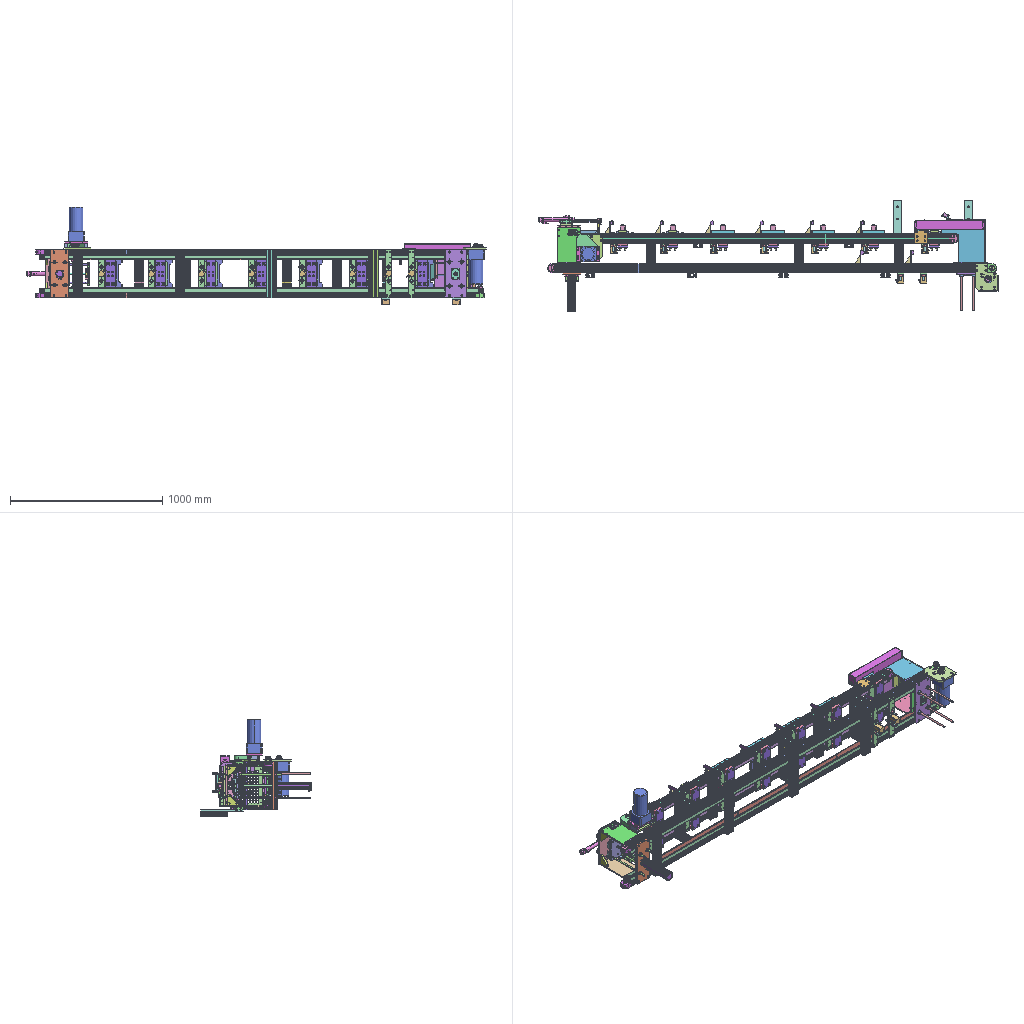Assembly | STEP file | 130 different items | 544 placed | box 3024 x 734 x 644 mm
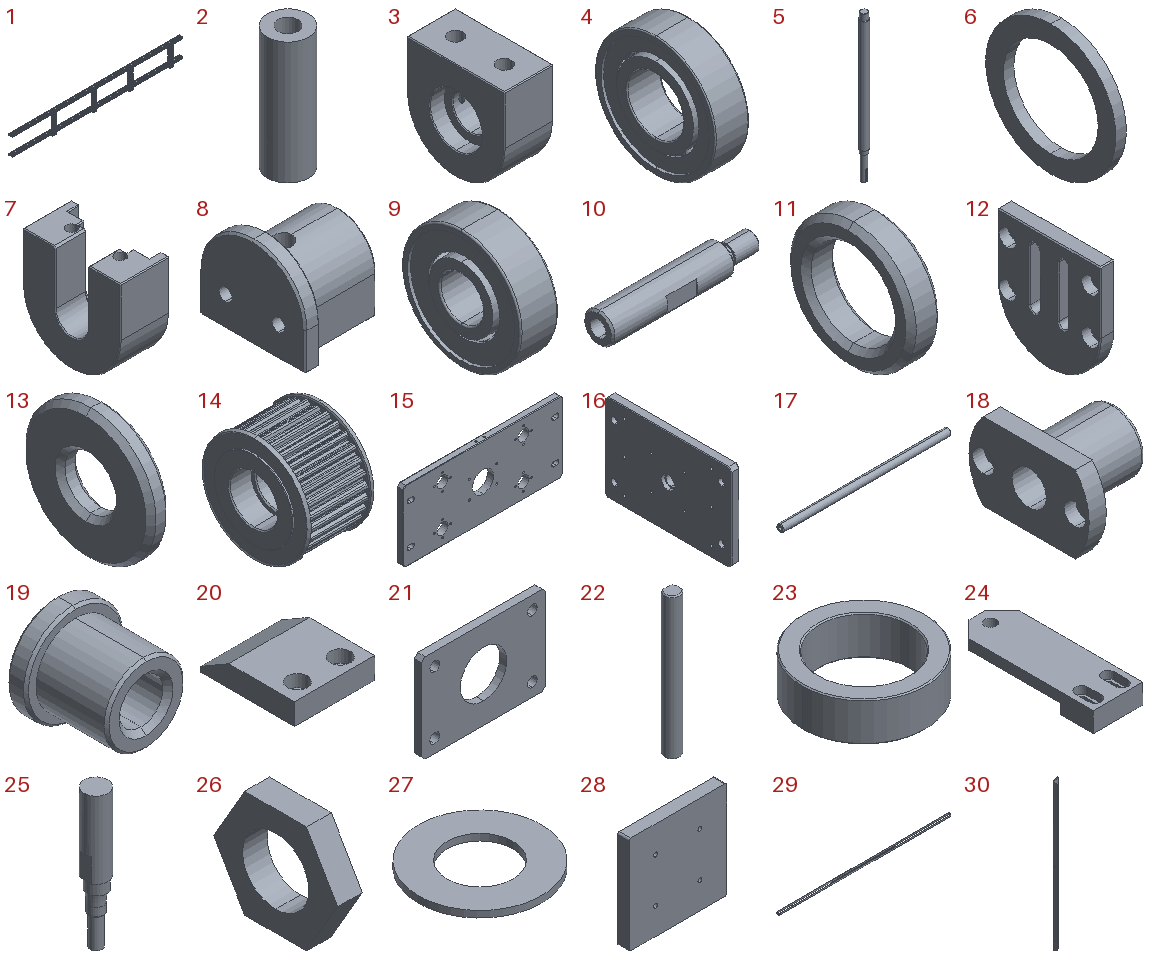Parts list (item | name | quantity | parent item | size | volume):
1 | Welding Conveyor Frame_Default<As Machined> | x1 | in BPSP-03Fixture Return Conveyor Assembly_Default | 2830 x 90 x 316 mm | 3898026 mm3
2 | DYCS-M-15-17 Threaded Bushing_Default | x16 | in BPSP-03Fixture Return Conveyor Assembly_Default, BPSP-02Welding Conveyor Assembly_Default | 10 x 10 x 30 mm | 1767 mm3
3 | BPSP-03-004 Elevator Drive Shaft Fixing Plate_Default | x4 | in BPSP-03Fixture Return Conveyor Assembly_Default, BPSP-02Welding Conveyor Assembly_Default | 30 x 60 x 60 mm | 72459 mm3
4 | GB/T276-94Deep Groove Ball Bearing6002-2Z | x4 | in BPSP-03Fixture Return Conveyor Assembly_Default, BPSP-02Welding Conveyor Assembly_Default | 9 x 32 x 32 mm | 3545 mm3
5 | BPSP-03-006 Drive Shaft_Default | x2 | in BPSP-03Fixture Return Conveyor Assembly_Default, BPSP-02Welding Conveyor Assembly_Default | 18 x 18 x 335 mm | 73475 mm3
6 | BPSP-03-005 Locating Ring_Default | x4 | in BPSP-03Fixture Return Conveyor Assembly_Default, BPSP-02Welding Conveyor Assembly_Default | 2 x 25 x 25 mm | 461.437 mm3
7 | BPSP-03-018 Driven Wheel Mounting Plate_Default | x4 | in Driven Wheel Assembly_Default | 30 x 60 x 60 mm | 50936 mm3
8 | BPSP-03-019 Driven Wheel Fixing Block_Default | x4 | in Driven Wheel Assembly_Default | 23 x 28 x 24 mm | 8364 mm3
9 | GB/T276-94Deep Groove Ball Bearing608-2Z | x8 | in Driven Wheel Assembly_Default | 7 x 22 x 22 mm | 1460 mm3
10 | BPSP-03-021 Fixed Shaft_Default | x4 | in Driven Wheel Assembly_Default | 40.5 x 8 x 8 mm | 1575 mm3
11 | BPSP-03-022 Driven Wheel Stop Washer_Default | x4 | in Driven Wheel Assembly_Default | 3 x 12 x 12 mm | 168.916 mm3
12 | BPSP-03-020 Clamp Block_Default | x4 | in Driven Wheel Assembly_Default | 7 x 50 x 55 mm | 14443 mm3
13 | BPSP-03-023 Driven Wheel Fixing Washer_Default | x4 | in Driven Wheel Assembly_Default | 2 x 13 x 13 mm | 208.696 mm3
14 | BPSP-03-032 T5Timing Pulley30 Tooth2 | x4 | in Driven Wheel Assembly_Default | 32 x 49 x 49 mm | 40684 mm3
15 | BPSP-03-012 Linear Bearing Mounting Plate_Default | x1 | in Elevator Lift Mechanism | 316 x 12 x 140 mm | 486609 mm3
16 | BPSP-03-013 Test Station Lift Plate_Default | x1 | in Elevator Lift Mechanism | 12 x 190 x 130 mm | 287114 mm3
17 | BPSP-03-016 Lift Chrome Rod_Default | x4 | in Elevator Lift Mechanism | 280 x 12 x 12 mm | 31385 mm3
18 | LHFC12_LHFC12 | x4 | in Elevator Lift Mechanism | 30 x 42 x 27 mm | 10763 mm3
19 | BPSP-03-039Lift Joint | x1 | in Elevator Lift Mechanism | 19.8 x 18 x 19.8 mm | 2819 mm3
20 | BPSP-03-015 Shaft Pivot Seat | x2 | in Elevator Lift Mechanism | 30 x 35 x 8 mm | 6950 mm3
21 | BPSP-03-038Support Cylinder Fixing Plate_Default | x1 | in Elevator Lift Mechanism | 70 x 4 x 50 mm | 11431 mm3
22 | BPSP-03-014 Sliding Rib_Default | x2 | in Elevator Lift Mechanism | 14 x 12 x 130 mm | 17958 mm3
23 | BPSP-03-037Lift Retaining Ring_Default | x1 | in Elevator Lift Mechanism | 22 x 22 x 7 mm | 1249 mm3
24 | BPSP-03-036Proximity Switch Mounting Plate | x1 | in Elevator Lift Mechanism | 30 x 85 x 12 mm | 16342 mm3
25 | E2E_X2D1_N_BASE | x1 | in Proximity SensorE2E_X2D1_N | 8 x 8 x 47 mm | 1680 mm3
26 | E2E_X2D1_N_NUT | x2 | in Proximity SensorE2E_X2D1_N | 3 x 15.011 x 13 mm | 288.278 mm3
27 | E2E_X2D1_N_WASHER | x1 | in Proximity SensorE2E_X2D1_N | 15 x 15 x 0.8 mm | 101.159 mm3
28 | Ejector Urethane Pad_Default | x1 | in Elevator Lift Mechanism | 110 x 13 x 110 mm | 155824 mm3
29 | Belt1-11^BPSP-03Fixture Return Conveyor Assembly_Default | x2 | in BPSP-03Fixture Return Conveyor Assembly_Default | 2922 x 49 x 25 mm | 294683 mm3
30 | BPSP-03-031Long Support Plate (Lower)_Default | x6 | in BPSP-03Fixture Return Conveyor Assembly_Default | 35 x 30 x 929.978 mm | 113908 mm3
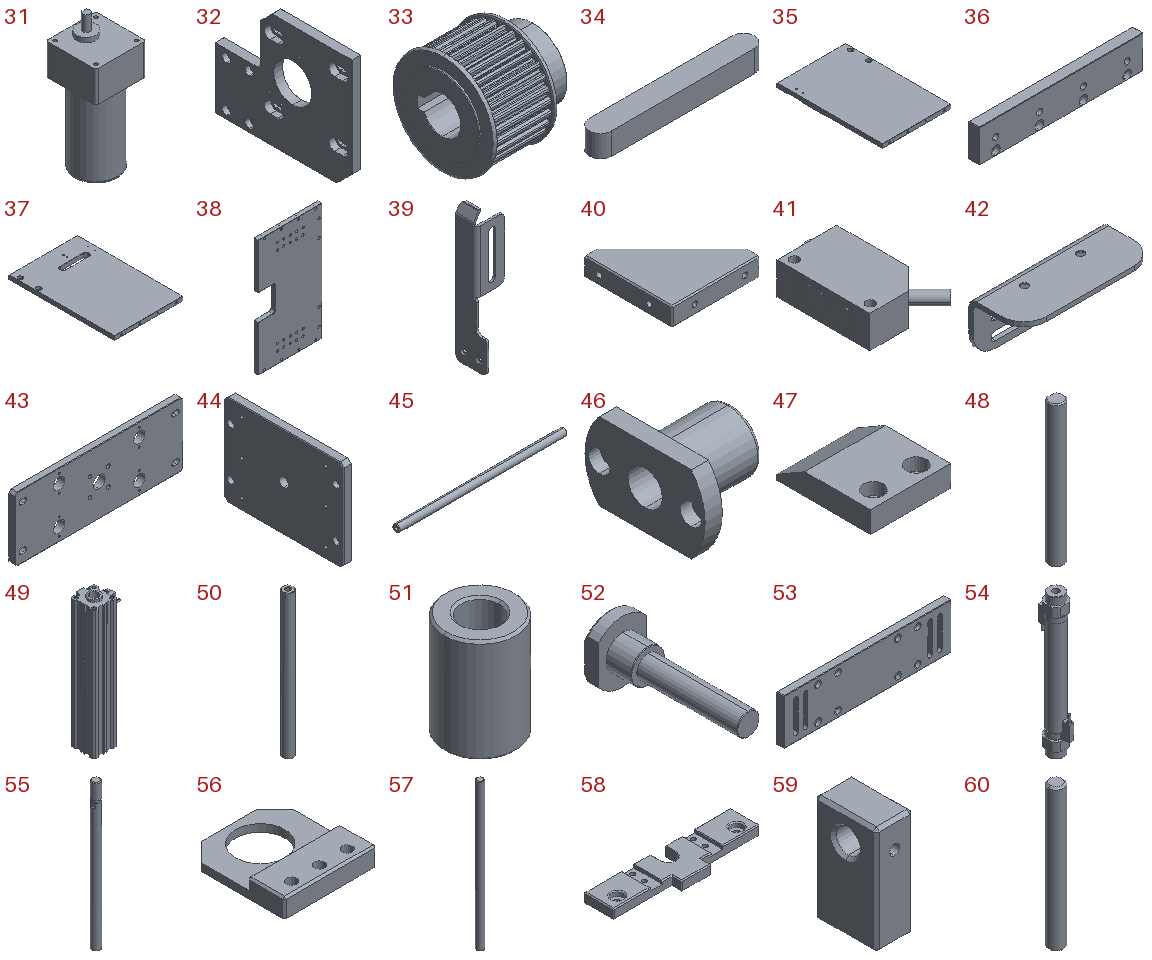31 | Taibang Reversible Motor90W_Default | x2 | in BPSP-03Fixture Return Conveyor Assembly_Default, Motor Assembly_Default | 104 x 104 x 269 mm | 1739193 mm3
32 | BPSP-03-011 Motor Fixing Plate2_Default | x1 | in BPSP-03Fixture Return Conveyor Assembly_Default | 12 x 180 x 150 mm | 230112 mm3
33 | BPSP-03-007 T5Timing Pulley30 Tooth1 | x4 | in BPSP-03Fixture Return Conveyor Assembly_Default, BPSP-02Welding Conveyor Assembly_Default | 44 x 49 x 49 mm | 49129 mm3
34 | BPSP-03-008 Flat Key_Default | x2 | in BPSP-03Fixture Return Conveyor Assembly_Default | 45 x 6 x 6 mm | 1574 mm3
35 | BPSP-11-002Unloading Support Plate1_Default | x1 | in BPSP-11Unloading Support Plate Assembly_Default | 150 x 230 x 9 mm | 307149 mm3
36 | BPSP-11-003Unloading Support Plate2_Default | x2 | in BPSP-11Unloading Support Plate Assembly_Default | 150 x 10 x 30 mm | 41531 mm3
37 | BPSP-11-001Unloading Support Plate_Default | x1 | in BPSP-11Unloading Support Plate Assembly_Default | 150 x 230 x 9 mm | 300493 mm3
38 | BPSP-11-004Unloading Support Plate3_Default | x1 | in BPSP-11Unloading Support Plate Assembly_Default | 150 x 10 x 274 mm | 378327 mm3
39 | BPSP-11-008Guide Plate_Default | x1 | in BPSP-11Unloading Support Plate Assembly_Default | 27 x 30 x 130 mm | 7946 mm3
40 | BPSP-11-006Reinforcing Rib_Default | x2 | in BPSP-11Unloading Support Plate Assembly_Default | 70 x 70 x 15 mm | 45416 mm3
41 | Photoelectric SensorE3Z_LS61 | x12 | in BPSP-11Unloading Support Plate Assembly_Default, CA-10Lift Stop Assembly_Default, Side Locating Sensor Assembly1_Default | 24.985 x 38.085 x 10.8 mm | 6465 mm3
42 | BPSP-L-17 Pull Sensor Mounting Plate_Default | x1 | in BPSP-11Unloading Support Plate Assembly_Default | 60 x 25 x 24 mm | 4566 mm3
43 | BPSP-11-17 Unloading Linear Bearing Mounting Plate_Default | x1 | in Elevator Lift Mechanism-2 | 316 x 12 x 120 mm | 422737 mm3
44 | BPSP-11-18 Unloading Lift Plate_Default | x1 | in Elevator Lift Mechanism-2 | 12 x 170 x 130 mm | 257545 mm3
45 | BPSP-03-016 Lift Chrome Rod-2_Default | x4 | in Elevator Lift Mechanism-2 | 280 x 12 x 12 mm | 31385 mm3
46 | LHFC12-2_LHFC12 | x4 | in Elevator Lift Mechanism-2 | 30 x 42 x 27 mm | 10763 mm3
47 | BPSP-03-015 Shaft Pivot Seat-2 | x2 | in Elevator Lift Mechanism-2 | 30 x 35 x 8 mm | 6950 mm3
48 | BPSP-03-014 Sliding Rib-2_Default | x2 | in Elevator Lift Mechanism-2 | 14 x 12 x 130 mm | 17958 mm3
49 | A_CDQ2A32-200DC-F7NV(0)_Default | x1 | in CDQ2A-200_Default | 63.2 x 49.5 x 249.5 mm | 394520 mm3
50 | A_CDQ2A32-200DC-F7NV(0) - Copy_Default | x1 | in Elevator Lift Mechanism-2 | 16 x 16 x 218 mm | 43283 mm3
51 | BPSP-11-19 Cylinder Extension Shaft_Default | x1 | in Elevator Lift Mechanism-2 | 16 x 16 x 23 mm | 3300 mm3
52 | BPSP-11-20 Cylinder Connection Shoulder Screw_Default | x1 | in Elevator Lift Mechanism-2 | 17 x 50.1 x 22 mm | 4480 mm3
53 | BPSP-11-09 Pusher Fixing Plate_Default | x1 | in Pusher Assembly_Default | 256 x 12 x 70 mm | 193349 mm3
54 | A_CDM2B25-150-C76(0)_Default | x1 | in CDM-25-150_Default | 30 x 52.6 x 238 mm | 131860 mm3
55 | A_CDM2B25-150-C76(1)_Default | x1 | in CDM-25-150_Default | 10 x 10 x 183 mm | 14238 mm3
56 | BPSP-11-10 Pusher Cylinder Fixing Plate_Default | x1 | in Pusher Assembly_Default | 50 x 55 x 10 mm | 13598 mm3
57 | BPSP-11-11 12Chrome Rod_Default | x2 | in Pusher Assembly_Default | 12 x 12 x 270 mm | 30254 mm3
58 | BPSP-11-13 Rotary Support Plate_Default | x1 | in Pusher Assembly_Default | 150 x 40 x 10 mm | 40974 mm3
59 | BPSP-11-14 Pusher Shaft Fixing Plate_Default | x2 | in Pusher Assembly_Default | 12 x 20 x 35 mm | 7342 mm3
60 | BPSP-11-15 10Rotating Shaft_Default | x1 | in Pusher Assembly_Default | 8 x 8 x 74 mm | 3697 mm3
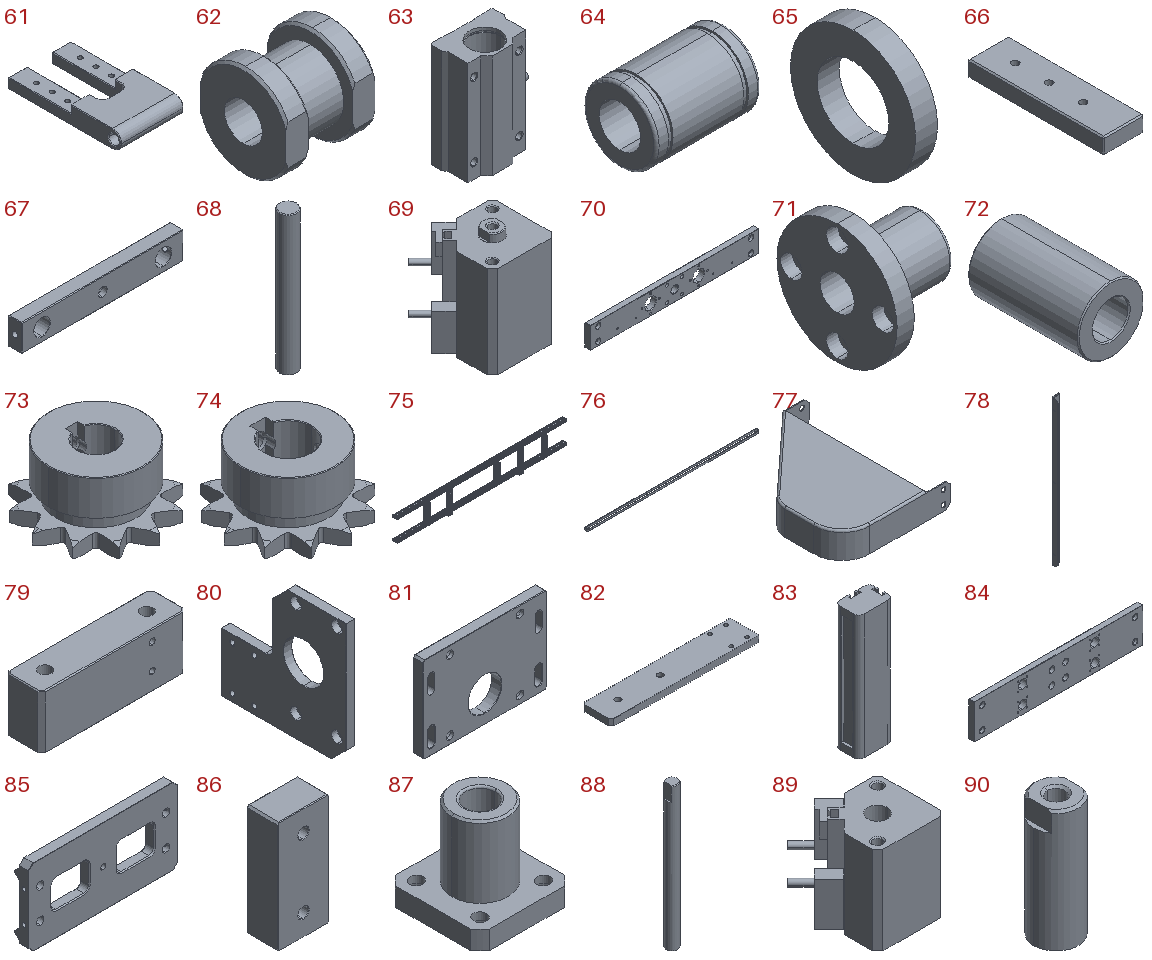61 | BPSP-11-16 Pusher Plate_Default | x1 | in Pusher Assembly_Default | 50 x 90 x 14 mm | 32757 mm3
62 | BPSP-11-12 Pusher Cylinder Connecting Block_Default | x1 | in Pusher Assembly_Default | 20 x 19 x 21 mm | 3951 mm3
63 | LHBBW12body_Default | x2 | in LHBBW12_LHBBW12, Pusher Assembly_Default | 49 x 28 x 70 mm | 46534 mm3
64 | LMU12_Default | x2 | in LHBBW12_LHBBW12 | 30 x 21 x 21 mm | 6896 mm3
65 | LHBBW12collar3_Default | x1 | in LHBBW12_LHBBW12 | 3.7 x 21 x 21 mm | 863.074 mm3
66 | BPSP-11-21 Bumper Block_Default | x2 | in Pusher Assembly_Default | 15 x 50 x 6 mm | 4377 mm3
67 | BPSP-L-07 Lift Connecting Plate_Default | x9 | in Universal Test Stopper12_Default | 120 x 10 x 20 mm | 20677 mm3
68 | BPSP-L-08 Test Guide Rod_Default | x18 | in Universal Test Stopper12_Default | 12 x 12 x 95 mm | 10735 mm3
69 | A_CDQ2A25-25D-F7NV012_Default | x9 | in Universal Test Stopper12_Default | 52.598 x 52.598 x 62.5 mm | 85379 mm3
70 | BPSP-L-06 Stopper Cylinder Mount | x9 | in Universal Test Stopper12_Default | 316 x 10 x 40 mm | 112914 mm3
71 | LHFR122_Default | x18 | in Universal Test Stopper12_Default | 30 x 42 x 42 mm | 12352 mm3
72 | BPSP-L-09 Lift Cylinder Extension Rod_Default | x9 | in Universal Test Stopper12_Default | 12 x 20 x 12 mm | 1596 mm3
73 | SP35B12_N_12_SP35B12-N-12 | x2 | in BPSP-03Fixture Return Conveyor Assembly_Default, BPSP-02Welding Conveyor Assembly_Default | 41 x 41 x 20 mm | 11740 mm3
74 | SP35B12_N_15_SP35B12-N-15 | x2 | in BPSP-03Fixture Return Conveyor Assembly_Default, Motor Assembly_Default | 41 x 41 x 20 mm | 10343 mm3
75 | Welding Conveyor Frame01_Default<As Machined> | x1 | in BPSP-02Welding Conveyor Assembly_Default | 2360 x 90 x 316 mm | 3445395 mm3
76 | Welding Process Conveyor Belt_Default | x2 | in BPSP-02Welding Conveyor Assembly_Default | 2454 x 51.95 x 25 mm | 495464 mm3
77 | BPSP-02-004 Guard | x1 | in BPSP-02Welding Conveyor Assembly_Default | 117 x 152.64 x 28 mm | 18137 mm3
78 | BPSP-02-014 Long Support Plate_Default | x6 | in BPSP-02Welding Conveyor Assembly_Default | 35 x 30 x 774.978 mm | 94609 mm3
79 | BPSP-02-003 Motor Post_Default | x2 | in Motor Assembly_Default | 80 x 20 x 30 mm | 45190 mm3
80 | BPSP-02-002 Motor Fixing Plate_Default | x1 | in Motor Assembly_Default | 12 x 170 x 170 mm | 228176 mm3
81 | 180WMotor Mounting Plate_Default | x1 | in Motor Assembly_Default | 150 x 12 x 104 mm | 156125 mm3
82 | BPSP-02-010 Light Curtain Mounting Bracket_Default | x2 | in BPSP-02Welding Conveyor Assembly_Default | 280 x 55 x 12 mm | 179701 mm3
83 | Light Curtain Sensor_Default | x2 | in BPSP-02Welding Conveyor Assembly_Default | 50 x 35 x 180 mm | 266071 mm3
84 | Lift Cylinder Fixing Bracket01 | x7 | in Fixture Lift Mechanism Assembly | 316 x 10 x 65 mm | 191391 mm3
85 | Lift Cylinder Fixing Bracket02 | x7 | in Fixture Lift Mechanism Assembly | 160 x 15 x 82 mm | 115095 mm3
86 | Lift Cylinder Fixing Bracket03 | x14 | in Fixture Lift Mechanism Assembly | 30 x 18 x 65 mm | 34026 mm3
87 | Linear BearingLMK8UU_Default | x28 | in Fixture Lift Mechanism Assembly | 25 x 25 x 24 mm | 4786 mm3
88 | Locating Guide Rod_Default | x28 | in Fixture Lift Mechanism Assembly | 8 x 8 x 100 mm | 4985 mm3
89 | CDQ2A20_15D_F7NV0 | x7 | in Fixture Lift Mechanism Assembly | 48.335 x 48.335 x 46.5 mm | 53480 mm3
90 | CDQ2A20_15D_1_F7NV0 | x7 | in Fixture Lift Mechanism Assembly | 10 x 10 x 27.5 mm | 2020 mm3
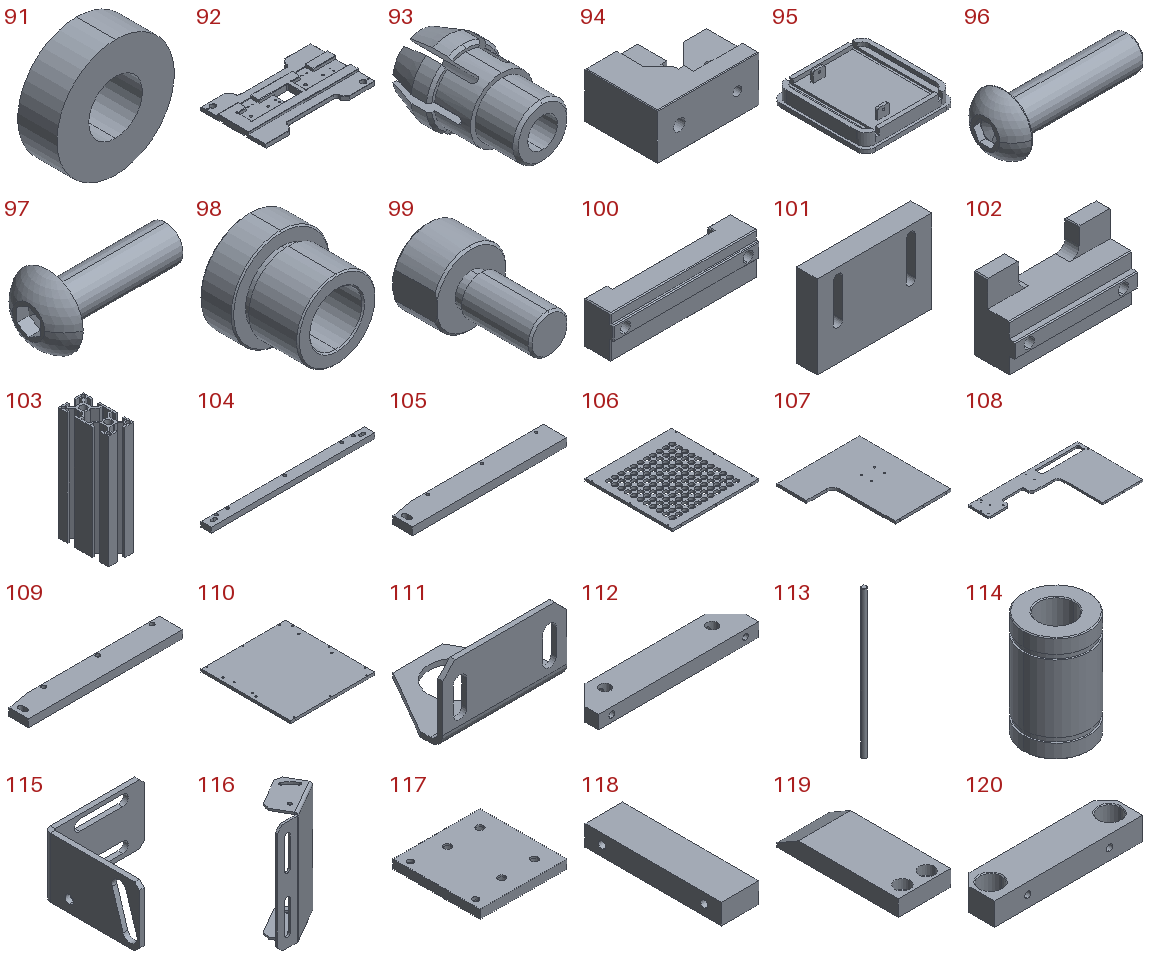91 | BPSP-L-20 Lift Mechanism Spacer Plate_Default | x7 | in Fixture Lift Mechanism Assembly | 12 x 4 x 12 mm | 357.356 mm3
92 | Bottom-Hole Locating Fixture Carrier Plate | x7 | in Experimental | 255 x 150 x 14 mm | 299894 mm3
93 | 8mmSpring Locating Pin | x14 | in Experimental | 8.161 x 13.5 x 8.2 mm | 235.099 mm3
94 | Product Fixture | x28 | in Product Fixture_Default, Experimental | 70 x 50 x 32 mm | 81575 mm3
95 | Product_Default | x12 | in Product Fixture_Default | 23 x 24 x 5.6 mm | 1586 mm3
96 | socket button head screw_iso_PreviewCfg | x7 | in Experimental | 68.8 x 28 x 28 mm | 15482 mm3
97 | hexagon socket button head screws gb_PreviewCfg | x7 | in Experimental | 23.3 x 12 x 12 mm | 775.96 mm3
98 | BPSP-L-01 Side Locating Guide Bushing_Default | x14 | in Experimental | 15 x 13.5 x 15 mm | 1145 mm3
99 | BPSP-L-05 Fixture Spacer Block_Default | x14 | in Experimental | 7 x 12.5 x 7.5 mm | 290.271 mm3
100 | BPSP-02-015 Fixture Locator V-Edge2-2_Default | x3 | in Product Clamp Locator Two-Piece Assembly_Default | 80 x 16 x 23 mm | 22056 mm3
101 | BPSP-02-016 Fixture Locator V-Edge1-2_Default | x3 | in Product Clamp Locator Two-Piece Assembly_Default | 55 x 10 x 40 mm | 20062 mm3
102 | BPSP-02-018 Fixture Locating Plate156 Station_Default | x3 | in BPSP-02Welding Conveyor Assembly_Default, Welding and Return Conveyor Assembly | 65 x 22 x 39 mm | 33983 mm3
103 | BPSP-03-003 Aluminium Profile01_Default<As Machined> | x6 | in Welding and Return Conveyor Assembly | 30 x 60 x 135 mm | 76001 mm3
104 | CA-10-005Lift Stop Plate1_Default | x1 | in CA-10Lift Stop Assembly_Default | 316 x 20 x 10 mm | 61183 mm3
105 | CA-10-006Lift Stop Plate2_Default | x1 | in CA-10Lift Stop Assembly_Default | 200 x 30 x 10 mm | 58212 mm3
106 | CA-10-007Lift Stop Plate3_Default | x1 | in CA-10Lift Stop Assembly_Default | 272 x 275 x 8 mm | 402632 mm3
107 | CA-10-009Lift Stop Plate5_Default | x1 | in CA-10Lift Stop Assembly_Default | 248 x 275 x 8 mm | 425355 mm3
108 | CA-10-008Lift Stop Plate4_Default | x1 | in CA-10Lift Stop Assembly_Default | 458 x 275 x 8 mm | 503075 mm3
109 | CA-10-020Lift Stop Plate2_Default | x1 | in CA-10Lift Stop Assembly_Default | 200 x 30 x 10 mm | 58212 mm3
110 | CA-10-010Lift Stop Plate6_Default | x1 | in CA-10Lift Stop Assembly_Default | 256 x 272 x 8 mm | 553953 mm3
111 | CA-10-017Cylinder Mount_Default | x2 | in CA-10Lift Stop Assembly_Default | 50 x 35 x 29 mm | 4191 mm3
112 | CA-10-011Pusher Base_Default | x2 | in CA-10Lift Stop Assembly_Default | 120 x 25 x 10 mm | 26219 mm3
113 | CA-10-012Pusher Rod_Default | x2 | in CA-10Lift Stop Assembly_Default | 8 x 8 x 240 mm | 11986 mm3
114 | Linear BearingLM8UU_Default | x4 | in CA-10Lift Stop Assembly_Default | 15 x 15 x 24 mm | 2996 mm3
115 | CA-10-001Sensor Mount_Default | x1 | in CA-10Lift Stop Assembly_Default | 40 x 40 x 25 mm | 3201 mm3
116 | CA-10-002Sensor Mounting Plate_Default | x1 | in CA-10Lift Stop Assembly_Default | 55.641 x 41.151 x 114 mm | 16325 mm3
117 | CA-10-003Lift Stop Fixing Plate_Default | x1 | in CA-10Lift Stop Assembly_Default | 80 x 80 x 8 mm | 47659 mm3
118 | CA-10-004Lift Stop Fixing Plate2_Default | x1 | in CA-10Lift Stop Assembly_Default | 22 x 80 x 12 mm | 20510 mm3
119 | CA-10-013Pusher Plate | x2 | in CA-10Lift Stop Assembly_Default | 26 x 60 x 8 mm | 11155 mm3
120 | CA-10-014Pusher Moving Plate_Default | x1 | in CA-10Lift Stop Assembly_Default | 100 x 25 x 15.3 mm | 31484 mm3
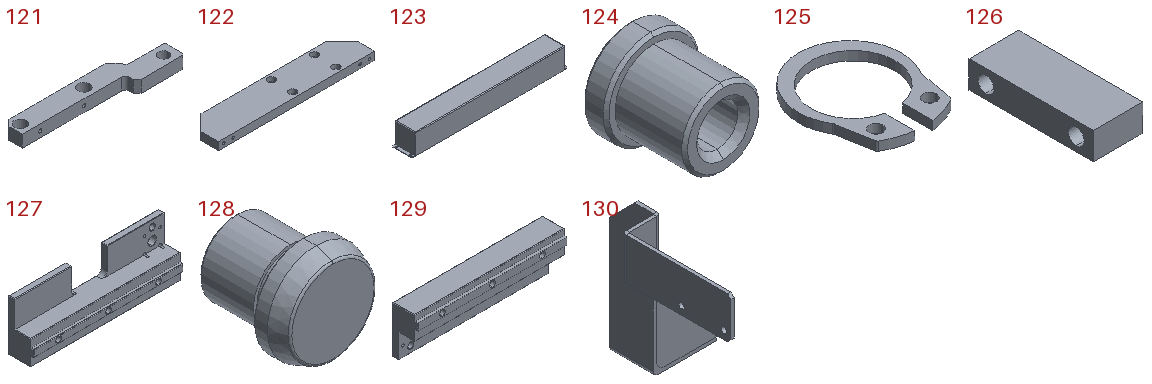121 | CA-10-015Pusher Moving Plate2_Default | x1 | in CA-10Lift Stop Assembly_Default | 190 x 40 x 15.3 mm | 65560 mm3
122 | CA-10-016Pusher Connecting Plate_Default | x1 | in CA-10Lift Stop Assembly_Default | 200 x 42 x 10 mm | 77675 mm3
123 | CA-10-018Cylinder Cover_Default | x1 | in CA-10Lift Stop Assembly_Default | 458 x 60 x 60 mm | 82593 mm3
124 | CA-10-019Floating Joint | x1 | in CA-10Lift Stop Assembly_Default | 15.8 x 15.5 x 15.8 mm | 1661 mm3
125 | circlips for shaft--type a large gb_PreviewCfg | x8 | in CA-10Lift Stop Assembly_Default | 11.5 x 13.997 x 1 mm | 50.603 mm3
126 | CA-10-021Light Curtain Support Plate_Default | x2 | in CA-10Lift Stop Assembly_Default | 22 x 55 x 12 mm | 12827 mm3
127 | BPSP-02-018 Fixture Locating Plate_Default | x4 | in Side Clamp Assembly_Default | 150 x 25 x 51 mm | 98863 mm3
128 | BPSP-L-03 Fixture Locating Pin_Default | x8 | in Side Clamp Assembly_Default, Product Clamp Locator V-Face Assembly_Default | 8 x 8 x 8 mm | 267.813 mm3
129 | BPSP-02-015 Fixture Locator V-Edge2_Default | x4 | in Product Clamp Locator V-Face Assembly_Default | 150 x 25 x 47 mm | 97185 mm3
130 | Sensor Mount2_Default | x8 | in Side Locating Sensor Assembly1_Default | 57.322 x 91.966 x 85 mm | 12045 mm3
Placements (level | parent | child | x y z in mm | rotation matrix by rows), first 180 of 616 lines:
1 | Welding and Return Conveyor Assembly | BPSP-03Fixture Return Conveyor Assembly_Default | -0.0 -0.0 -0.0 | 1 0 0 0 1 0 0 0 1
2 | BPSP-03Fixture Return Conveyor Assembly_Default | Welding Conveyor Frame_Default<As Machined> | -0.0 -0.0 -0.0 | -1 0 0 0 1 0 0 0 -1
2 | BPSP-03Fixture Return Conveyor Assembly_Default | DYCS-M-15-17 Threaded Bushing_Default | 1385.0 15.0 -143.0 | 0 0 1 0 1 0 -1 0 0
2 | BPSP-03Fixture Return Conveyor Assembly_Default | DYCS-M-15-17 Threaded Bushing_Default | 1385.0 -15.0 -143.0 | 0 0 1 0.9242 -0.3818 0 0.3818 0.9242 0
2 | BPSP-03Fixture Return Conveyor Assembly_Default | DYCS-M-15-17 Threaded Bushing_Default | -1415.0 -15.0 143.0 | 0 0 1 0.007845 1 0 -1 0.007845 0
2 | BPSP-03Fixture Return Conveyor Assembly_Default | DYCS-M-15-17 Threaded Bushing_Default | -1415.0 15.0 143.0 | 0 0 1 0 1 0 -1 0 0
2 | BPSP-03Fixture Return Conveyor Assembly_Default | DYCS-M-15-17 Threaded Bushing_Default | -1415.0 15.0 -143.0 | 0 0 1 0 1 0 -1 0 0
2 | BPSP-03Fixture Return Conveyor Assembly_Default | DYCS-M-15-17 Threaded Bushing_Default | -1415.0 -15.0 -143.0 | 0 0 1 0 1 0 -1 0 0
2 | BPSP-03Fixture Return Conveyor Assembly_Default | DYCS-M-15-17 Threaded Bushing_Default | 1385.0 -15.0 143.0 | 0 0 1 0 1 0 -1 0 0
2 | BPSP-03Fixture Return Conveyor Assembly_Default | DYCS-M-15-17 Threaded Bushing_Default | 1385.0 15.0 143.0 | 0 0 1 0 1 0 -1 0 0
2 | BPSP-03Fixture Return Conveyor Assembly_Default | BPSP-03-004 Elevator Drive Shaft Fixing Plate_Default | 1430.0 -0.0 -128.0 | 0 0 -1 0 -1 0 -1 0 0
2 | BPSP-03Fixture Return Conveyor Assembly_Default | BPSP-03-004 Elevator Drive Shaft Fixing Plate_Default | 1430.0 -0.0 128.0 | 0 0 -1 0 1 0 1 0 0
2 | BPSP-03Fixture Return Conveyor Assembly_Default | GB/T276-94Deep Groove Ball Bearing6002-2Z | 1445.0 -0.0 132.5 | 0 -0.9907 0.1358 0 -0.1358 -0.9907 1 0 -0
2 | BPSP-03Fixture Return Conveyor Assembly_Default | GB/T276-94Deep Groove Ball Bearing6002-2Z | 1445.0 -0.0 -132.5 | 0 0 -1 0 1 0 1 0 0
2 | BPSP-03Fixture Return Conveyor Assembly_Default | BPSP-03-006 Drive Shaft_Default | 1445.0 -0.0 -142.0 | -0.2677 0.9635 0 0.9635 0.2677 0 0 0 -1
2 | BPSP-03Fixture Return Conveyor Assembly_Default | BPSP-03-005 Locating Ring_Default | 1445.0 -0.0 126.0 | 0 0 -1 0 1 0 1 0 0
2 | BPSP-03Fixture Return Conveyor Assembly_Default | BPSP-03-005 Locating Ring_Default | 1445.0 -0.0 -128.0 | 0 0 -1 0 1 0 1 0 0
2 | BPSP-03Fixture Return Conveyor Assembly_Default | Driven Wheel Assembly_Default | -1430.0 -0.0 128.0 | 0 0 1 0 -1 0 1 0 0
3 | Driven Wheel Assembly_Default | BPSP-03-018 Driven Wheel Mounting Plate_Default | -0.0 -0.0 -0.0 | 1 0 0 0 1 0 0 0 1
3 | Driven Wheel Assembly_Default | BPSP-03-019 Driven Wheel Fixing Block_Default | 23.0 0.0 15.0 | -1 0 0 0 1 0 0 0 -1
3 | Driven Wheel Assembly_Default | GB/T276-94Deep Groove Ball Bearing608-2Z | -27.5 -0.0 2.73 | 1 0 0 0 -0.000286 -1 0 1 -0.000286
3 | Driven Wheel Assembly_Default | BPSP-03-021 Fixed Shaft_Default | -32.5 0.0 2.73 | 1 0 0 0 -1 0 0 0 -1
3 | Driven Wheel Assembly_Default | GB/T276-94Deep Groove Ball Bearing608-2Z | -6.5 -0.0 2.73 | -1 0 0 0 -0.9992 0.03909 0 0.03909 0.9992
3 | Driven Wheel Assembly_Default | BPSP-03-022 Driven Wheel Stop Washer_Default | -0.0 0.0 2.73 | -1 0 0 0 0.1471 -0.9891 0 -0.9891 -0.1471
3 | Driven Wheel Assembly_Default | BPSP-03-020 Clamp Block_Default | 30.0 -0.0 15.0 | -1 0 0 0 -1 0 0 0 1
3 | Driven Wheel Assembly_Default | BPSP-03-023 Driven Wheel Fixing Washer_Default | -33.0 -0.0 2.73 | 1 0 0 0 0.9757 0.2192 0 -0.2192 0.9757
3 | Driven Wheel Assembly_Default | BPSP-03-032 T5Timing Pulley30 Tooth2 | -34.0 -0.0 2.73 | 1 0 0 0 1 0 0 0 1
2 | BPSP-03Fixture Return Conveyor Assembly_Default | Driven Wheel Assembly_Default | -1430.0 -0.0 -128.0 | 0 0 1 0 1 0 -1 0 -0
3 | Driven Wheel Assembly_Default | BPSP-03-018 Driven Wheel Mounting Plate_Default | -0.0 -0.0 -0.0 | 1 0 0 0 1 0 0 0 1
3 | Driven Wheel Assembly_Default | BPSP-03-019 Driven Wheel Fixing Block_Default | 23.0 0.0 15.0 | -1 0 0 0 1 0 0 0 -1
3 | Driven Wheel Assembly_Default | GB/T276-94Deep Groove Ball Bearing608-2Z | -27.5 -0.0 2.73 | 1 0 0 0 -0.000286 -1 0 1 -0.000286
3 | Driven Wheel Assembly_Default | BPSP-03-021 Fixed Shaft_Default | -32.5 0.0 2.73 | 1 0 0 0 -1 0 0 0 -1
3 | Driven Wheel Assembly_Default | GB/T276-94Deep Groove Ball Bearing608-2Z | -6.5 -0.0 2.73 | -1 0 0 0 -0.9992 0.03909 0 0.03909 0.9992
3 | Driven Wheel Assembly_Default | BPSP-03-022 Driven Wheel Stop Washer_Default | -0.0 0.0 2.73 | -1 0 0 0 0.1471 -0.9891 0 -0.9891 -0.1471
3 | Driven Wheel Assembly_Default | BPSP-03-020 Clamp Block_Default | 30.0 -0.0 15.0 | -1 0 0 0 -1 0 0 0 1
3 | Driven Wheel Assembly_Default | BPSP-03-023 Driven Wheel Fixing Washer_Default | -33.0 -0.0 2.73 | 1 0 0 0 0.9757 0.2192 0 -0.2192 0.9757
3 | Driven Wheel Assembly_Default | BPSP-03-032 T5Timing Pulley30 Tooth2 | -34.0 -0.0 2.73 | 1 0 0 0 1 0 0 0 1
2 | BPSP-03Fixture Return Conveyor Assembly_Default | Elevator Lift Mechanism | 1288.35 13.745 -33.168 | 0 0 -1 0 1 0 1 0 0
3 | Elevator Lift Mechanism | BPSP-03-012 Linear Bearing Mounting Plate_Default | 33.168 -55.745 3.35 | 1 0 0 0 1 0 0 0 1
3 | Elevator Lift Mechanism | BPSP-03-013 Test Station Lift Plate_Default | 33.168 -1.645 3.35 | 0 1 0 -1 0 0 0 0 1
3 | Elevator Lift Mechanism | BPSP-03-016 Lift Chrome Rod_Default | 113.168 -13.645 -36.65 | 0 0.9719 0.2354 -1 0 0 0 -0.2354 0.9719
3 | Elevator Lift Mechanism | BPSP-03-016 Lift Chrome Rod_Default | 113.168 -13.645 43.35 | 0 0.6574 -0.7536 -1 0 0 0 0.7536 0.6574
3 | Elevator Lift Mechanism | LHFC12_LHFC12 | 113.168 -37.745 -36.65 | 0 1 0 -1 0 0 0 0 1
3 | Elevator Lift Mechanism | LHFC12_LHFC12 | 113.168 -37.745 43.35 | 0 1 0 -1 0 0 0 0 1
3 | Elevator Lift Mechanism | BPSP-03-039Lift Joint | 33.168 -20.745 3.35 | 1 0 0 0 1 0 0 0 1
3 | Elevator Lift Mechanism | BPSP-03-015 Shaft Pivot Seat | 3.168 -7.645 -65.65 | -1 0 0 0 1 0 0 0 -1
3 | Elevator Lift Mechanism | BPSP-03-038Support Cylinder Fixing Plate_Default | 33.168 -55.745 3.35 | 1 0 0 0 1 0 0 0 1
3 | Elevator Lift Mechanism | LHFC12_LHFC12 | -46.832 -37.745 -36.65 | 0 1 0 -1 0 0 0 0 1
3 | Elevator Lift Mechanism | LHFC12_LHFC12 | -46.832 -37.745 43.35 | 0 1 0 -1 0 0 0 0 1
3 | Elevator Lift Mechanism | BPSP-03-016 Lift Chrome Rod_Default | -46.832 -13.645 43.35 | 0 0.6574 -0.7536 -1 0 0 0 0.7536 0.6574
3 | Elevator Lift Mechanism | BPSP-03-016 Lift Chrome Rod_Default | -46.832 -13.645 -36.65 | 0 0.6574 -0.7536 -1 0 0 0 0.7536 0.6574
3 | Elevator Lift Mechanism | BPSP-03-015 Shaft Pivot Seat | 63.168 -7.645 -65.65 | -1 0 0 0 1 0 0 0 -1
3 | Elevator Lift Mechanism | BPSP-03-014 Sliding Rib_Default | -31.832 3.355 68.35 | 1 0 0 0 -1 0 0 0 -1
3 | Elevator Lift Mechanism | BPSP-03-014 Sliding Rib_Default | 98.168 3.355 68.35 | 1 0 0 0 -1 0 0 0 -1
3 | Elevator Lift Mechanism | BPSP-03-037Lift Retaining Ring_Default | 33.168 -17.145 3.35 | 1 0 0 0 0 1 0 -1 -0
3 | Elevator Lift Mechanism | BPSP-03-036Proximity Switch Mounting Plate | 33.168 -49.745 -72.65 | -1 0 0 0 1 0 0 0 -1
3 | Elevator Lift Mechanism | Proximity SensorE2E_X2D1_N | 33.168 21.255 -61.65 | 1 0 0 0 1 0 0 0 1
4 | Proximity SensorE2E_X2D1_N | E2E_X2D1_N_BASE | -0.0 -0.0 0.0 | 1 0 0 0 1 0 0 0 1
4 | Proximity SensorE2E_X2D1_N | E2E_X2D1_N_NUT | -0.0 -0.0 -11.0 | 0 0 -1 0 1 0 1 0 0
4 | Proximity SensorE2E_X2D1_N | E2E_X2D1_N_NUT | -0.0 -0.0 -16.8 | 0 0 -1 0 1 0 1 0 0
4 | Proximity SensorE2E_X2D1_N | E2E_X2D1_N_WASHER | -0.0 -0.0 -13.0 | 1 0 0 0 1 0 0 0 1
3 | Elevator Lift Mechanism | Ejector Urethane Pad_Default | 33.168 -1.645 3.35 | 1 0 0 0 1 0 0 0 1
2 | BPSP-03Fixture Return Conveyor Assembly_Default | Belt1-11^BPSP-03Fixture Return Conveyor Assembly_Default | 1445.73 -0.0 -97.5 | -1 0 0 0 -1 0 0 0 1
2 | BPSP-03Fixture Return Conveyor Assembly_Default | Belt1-11^BPSP-03Fixture Return Conveyor Assembly_Default | 1445.73 -0.0 122.5 | -1 0 0 0 -1 0 0 0 1
2 | BPSP-03Fixture Return Conveyor Assembly_Default | BPSP-03-031Long Support Plate (Lower)_Default | 993.236 15.0 -110.5 | 0 0 -1 0 1 0 1 0 0
2 | BPSP-03Fixture Return Conveyor Assembly_Default | BPSP-03-031Long Support Plate (Lower)_Default | 920.0 15.0 110.5 | 0 0 1 0 1 0 -1 0 -0
2 | BPSP-03Fixture Return Conveyor Assembly_Default | Taibang Reversible Motor90W_Default | 1420.0 -90.0 93.0 | 1 0 0 0 1 0 0 0 1
2 | BPSP-03Fixture Return Conveyor Assembly_Default | BPSP-03-011 Motor Fixing Plate2_Default | 1410.0 -60.0 170.0 | 0 0 1 0 1 0 -1 0 -0
2 | BPSP-03Fixture Return Conveyor Assembly_Default | BPSP-03-031Long Support Plate (Lower)_Default | 0.0 15.0 110.5 | 0 0 1 0 1 0 -1 0 -0
2 | BPSP-03Fixture Return Conveyor Assembly_Default | BPSP-03-031Long Support Plate (Lower)_Default | -920.0 15.0 110.5 | 0 0 1 0 1 0 -1 0 -0
2 | BPSP-03Fixture Return Conveyor Assembly_Default | BPSP-03-031Long Support Plate (Lower)_Default | 73.236 15.0 -110.5 | 0 0 -1 0 1 0 1 0 0
2 | BPSP-03Fixture Return Conveyor Assembly_Default | BPSP-03-031Long Support Plate (Lower)_Default | -846.764 15.0 -110.5 | 0 0 -1 0 1 0 1 0 0
2 | BPSP-03Fixture Return Conveyor Assembly_Default | BPSP-03-007 T5Timing Pulley30 Tooth1 | 1445.0 -0.0 126.0 | 0 0.9635 0.2677 0 0.2677 -0.9635 -1 0 0
2 | BPSP-03Fixture Return Conveyor Assembly_Default | BPSP-03-007 T5Timing Pulley30 Tooth1 | 1445.0 -0.0 -126.0 | 0 0.9635 -0.2677 0 0.2677 0.9635 1 0 -0
2 | BPSP-03Fixture Return Conveyor Assembly_Default | BPSP-03-008 Flat Key_Default | 1453.19 2.275 102.5 | 0 -0.2677 -0.9635 0 0.9635 -0.2677 1 0 0
2 | BPSP-03Fixture Return Conveyor Assembly_Default | BPSP-03-008 Flat Key_Default | 1453.19 2.275 -103.5 | 0 -0.2677 -0.9635 0 0.9635 -0.2677 1 0 0
2 | BPSP-03Fixture Return Conveyor Assembly_Default | BPSP-11Unloading Support Plate Assembly_Default | -1335.0 155.0 -128.0 | -1 0 0 0 1 0 0 0 -1
3 | BPSP-11Unloading Support Plate Assembly_Default | BPSP-11-002Unloading Support Plate1_Default | -0.0 -0.0 -0.0 | 1 0 0 0 1 0 0 0 1
3 | BPSP-11Unloading Support Plate Assembly_Default | BPSP-11-003Unloading Support Plate2_Default | -0.0 -125.0 15.0 | 1 0 0 0 1 0 0 0 1
3 | BPSP-11Unloading Support Plate Assembly_Default | BPSP-11-001Unloading Support Plate_Default | -0.0 -0.0 -256.0 | -1 0 0 0 1 0 0 0 -1
3 | BPSP-11Unloading Support Plate Assembly_Default | BPSP-11-003Unloading Support Plate2_Default | 0.0 -125.0 -271.0 | -1 0 0 0 1 0 0 0 -1
3 | BPSP-11Unloading Support Plate Assembly_Default | BPSP-11-004Unloading Support Plate3_Default | -0.0 115.0 -128.0 | 1 0 0 0 1 0 0 0 1
3 | BPSP-11Unloading Support Plate Assembly_Default | BPSP-11-008Guide Plate_Default | -70.0 75.0 1.8 | 0 0 -1 0 1 0 1 0 -0
3 | BPSP-11Unloading Support Plate Assembly_Default | BPSP-11-006Reinforcing Rib_Default | 60.0 80.0 -35.0 | 0 0 1 -1 0 0 0 -1 -0
3 | BPSP-11Unloading Support Plate Assembly_Default | BPSP-11-006Reinforcing Rib_Default | 75.0 80.0 -221.0 | 0 0 -1 -1 0 0 0 1 0
3 | BPSP-11Unloading Support Plate Assembly_Default | Photoelectric SensorE3Z_LS61 | -36.179 69.0 -273.0 | 0 1 0 0 0 -1 -1 0 0
3 | BPSP-11Unloading Support Plate Assembly_Default | BPSP-L-17 Pull Sensor Mounting Plate_Default | -23.479 74.4 -277.5 | 1 0 0 0 0 -1 0 1 0
2 | BPSP-03Fixture Return Conveyor Assembly_Default | Elevator Lift Mechanism-2 | -1320.35 13.745 33.168 | 0 0 1 0 1 0 -1 0 0
3 | Elevator Lift Mechanism-2 | BPSP-11-17 Unloading Linear Bearing Mounting Plate_Default | 33.168 -55.745 3.35 | 1 0 0 0 1 0 0 0 1
3 | Elevator Lift Mechanism-2 | BPSP-11-18 Unloading Lift Plate_Default | 33.168 193.255 3.35 | 0 1 0 -1 0 0 0 0 1
3 | Elevator Lift Mechanism-2 | BPSP-03-016 Lift Chrome Rod-2_Default | 108.168 181.255 -31.65 | 0 0.8804 0.4742 -1 0 0 0 -0.4742 0.8804
3 | Elevator Lift Mechanism-2 | BPSP-03-016 Lift Chrome Rod-2_Default | 108.168 181.255 38.35 | 0 0.6574 -0.7536 -1 0 0 0 0.7536 0.6574
3 | Elevator Lift Mechanism-2 | LHFC12-2_LHFC12 | 108.168 -37.745 -31.65 | 0 0 1 -1 0 0 0 -1 -0
3 | Elevator Lift Mechanism-2 | LHFC12-2_LHFC12 | 108.168 -37.745 38.35 | 0 0 1 -1 0 0 0 -1 0
3 | Elevator Lift Mechanism-2 | BPSP-03-015 Shaft Pivot Seat-2 | 3.168 187.255 -65.65 | -1 0 0 0 1 0 0 0 -1
3 | Elevator Lift Mechanism-2 | LHFC12-2_LHFC12 | -41.832 -37.745 -31.65 | 0 0 -1 -1 0 0 0 1 -0
3 | Elevator Lift Mechanism-2 | LHFC12-2_LHFC12 | -41.832 -37.745 38.35 | 0 0 -1 -1 0 0 0 1 -0
3 | Elevator Lift Mechanism-2 | BPSP-03-016 Lift Chrome Rod-2_Default | -41.832 181.255 38.35 | 0 0.897 0.442 -1 0 0 0 -0.442 0.897
3 | Elevator Lift Mechanism-2 | BPSP-03-016 Lift Chrome Rod-2_Default | -41.832 181.255 -31.65 | 0 0.6574 -0.7536 -1 0 0 0 0.7536 0.6574
3 | Elevator Lift Mechanism-2 | BPSP-03-015 Shaft Pivot Seat-2 | 63.168 187.255 -65.65 | -1 0 0 0 1 0 0 0 -1
3 | Elevator Lift Mechanism-2 | BPSP-03-014 Sliding Rib-2_Default | -26.832 198.255 68.35 | 1 0 0 0 -1 0 0 0 -1
3 | Elevator Lift Mechanism-2 | BPSP-03-014 Sliding Rib-2_Default | 93.168 198.255 68.35 | 1 0 0 0 -1 0 0 0 -1
3 | Elevator Lift Mechanism-2 | CDQ2A-200_Default | 33.168 -55.745 3.35 | 1 0 0 0 0 1 0 -1 0
4 | CDQ2A-200_Default | A_CDQ2A32-200DC-F7NV(0)_Default | -0.0 0.0 -0.0 | 1 0 0 0 1 0 0 0 1
3 | Elevator Lift Mechanism-2 | A_CDQ2A32-200DC-F7NV(0) - Copy_Default | 33.168 144.255 3.35 | 0.9055 0.4242 0 0 0 1 0.4242 -0.9055 0
3 | Elevator Lift Mechanism-2 | BPSP-11-19 Cylinder Extension Shaft_Default | 33.168 184.255 3.35 | 1 0 0 0 0 -1 0 1 -0
3 | Elevator Lift Mechanism-2 | BPSP-11-20 Cylinder Connection Shoulder Screw_Default | 33.168 148.155 3.35 | 1 0 0 0 1 0 0 0 1
2 | BPSP-03Fixture Return Conveyor Assembly_Default | Pusher Assembly_Default | -1355.377 280.0 0.0 | 0 0 -1 0 1 0 1 0 0
3 | Pusher Assembly_Default | BPSP-11-09 Pusher Fixing Plate_Default | -0.0 -0.0 -0.0 | 1 0 0 0 1 0 0 0 1
3 | Pusher Assembly_Default | CDM-25-150_Default | 0.0 38.0 -54.0 | -0.9991 -0.04323 0 -0.04323 0.9991 0 0 0 -1
4 | CDM-25-150_Default | A_CDM2B25-150-C76(0)_Default | 0.0 -0.0 -0.0 | 1 0 0 0 1 0 0 0 1
4 | CDM-25-150_Default | A_CDM2B25-150-C76(1)_Default | -0.0 0.0 150.0 | 1 0 0 0 1 0 0 0 1
3 | Pusher Assembly_Default | BPSP-11-10 Pusher Cylinder Fixing Plate_Default | 0.0 27.5 -45.0 | 1 0 0 0 1 0 0 0 1
3 | Pusher Assembly_Default | BPSP-11-11 12Chrome Rod_Default | 61.0 27.0 -226.0 | 0.9706 -0.2405 0 0.2405 0.9706 0 0 0 1
3 | Pusher Assembly_Default | BPSP-11-11 12Chrome Rod_Default | -61.0 28.0 -226.0 | -0.7326 0.6807 0 -0.6807 -0.7326 0 0 0 1
3 | Pusher Assembly_Default | BPSP-11-13 Rotary Support Plate_Default | 0.0 28.0 -231.0 | 1 0 0 0 1 0 0 0 1
3 | Pusher Assembly_Default | BPSP-11-14 Pusher Shaft Fixing Plate_Default | 31.0 30.5 -204.0 | -1 0 0 0 0 -1 0 -1 0
3 | Pusher Assembly_Default | BPSP-11-14 Pusher Shaft Fixing Plate_Default | -31.0 30.5 -204.0 | -1 0 0 0 0 -1 0 -1 0
3 | Pusher Assembly_Default | BPSP-11-15 10Rotating Shaft_Default | -36.962 21.5 -214.0 | 0 0 -1 0 1 0 1 0 -0
3 | Pusher Assembly_Default | BPSP-11-16 Pusher Plate_Default | 0.0 -17.292 -205.925 | 1 0 0 0 -0.9996 -0.02763 0 0.02763 -0.9996
3 | Pusher Assembly_Default | BPSP-11-12 Pusher Cylinder Connecting Block_Default | 0.0 38.0 -236.0 | 0 0.9977 0.06756 0 -0.06756 0.9977 1 0 -0
3 | Pusher Assembly_Default | LHBBW12_LHBBW12 | -61.0 27.0 -0.0 | -1 0 0 0 -1 0 0 0 1
4 | LHBBW12_LHBBW12 | LHBBW12body_Default | -0.0 -0.0 0.0 | 1 0 0 0 1 0 0 0 1
4 | LHBBW12_LHBBW12 | LMU12_Default | -0.0 -1.0 1.85 | 0 0 -1 0 1 0 1 0 -0
4 | LHBBW12_LHBBW12 | LMU12_Default | -0.0 -1.0 -31.85 | 0 0 -1 0 1 0 1 0 -0
4 | LHBBW12_LHBBW12 | LHBBW12collar3_Default | -0.0 -1.0 0.0 | 0 0 -1 0 1 0 1 0 -0
3 | Pusher Assembly_Default | LHBBW12body_Default | 61.0 27.0 -0.0 | -1 0 0 0 -1 0 0 0 1
3 | Pusher Assembly_Default | BPSP-11-21 Bumper Block_Default | 17.5 -37.671 -219.367 | 1 0 0 0 0.9996 0.02763 0 -0.02763 0.9996
3 | Pusher Assembly_Default | BPSP-11-21 Bumper Block_Default | -17.5 -37.671 -219.367 | 1 0 0 0 0.9996 0.02763 0 -0.02763 0.9996
2 | BPSP-03Fixture Return Conveyor Assembly_Default | Universal Test Stopper12_Default | 843.25 19.522 -1.088 | 0 0 -1 0 1 0 1 0 0
3 | Universal Test Stopper12_Default | BPSP-L-07 Lift Connecting Plate_Default | 1.088 -34.522 -1.75 | 1 0 0 0 1 0 0 0 1
3 | Universal Test Stopper12_Default | BPSP-L-08 Test Guide Rod_Default | 46.088 -7.522 -1.75 | -0.03222 -0.9995 0 0 0 -1 0.9995 -0.03222 -0
3 | Universal Test Stopper12_Default | BPSP-L-08 Test Guide Rod_Default | -43.912 -7.522 -1.75 | -0.1831 -0.9831 0 0 0 -1 0.9831 -0.1831 0
3 | Universal Test Stopper12_Default | A_CDQ2A25-25D-F7NV012_Default | 1.088 -59.522 -1.75 | -0.008539 -1 0 0 0 1 -1 0.008539 0
3 | Universal Test Stopper12_Default | BPSP-L-06 Stopper Cylinder Mount | 1.088 -59.522 -1.75 | 1 0 0 0 1 0 0 0 1
3 | Universal Test Stopper12_Default | LHFR122_Default | 46.088 -43.522 -1.75 | 0 1 0 -1 0 0 0 0 1
3 | Universal Test Stopper12_Default | LHFR122_Default | -43.912 -43.522 -1.75 | 0 0 -1 -1 0 0 0 1 0
3 | Universal Test Stopper12_Default | BPSP-L-09 Lift Cylinder Extension Rod_Default | 1.088 -54.522 -1.75 | 1 0 0 0 1 0 0 0 1
2 | BPSP-03Fixture Return Conveyor Assembly_Default | Universal Test Stopper12_Default | 993.25 19.522 -1.088 | 0 0 -1 0 1 0 1 0 0
3 | Universal Test Stopper12_Default | BPSP-L-07 Lift Connecting Plate_Default | 1.088 -34.522 -1.75 | 1 0 0 0 1 0 0 0 1
3 | Universal Test Stopper12_Default | BPSP-L-08 Test Guide Rod_Default | 46.088 -7.522 -1.75 | -0.03222 -0.9995 0 0 0 -1 0.9995 -0.03222 -0
3 | Universal Test Stopper12_Default | BPSP-L-08 Test Guide Rod_Default | -43.912 -7.522 -1.75 | -0.1831 -0.9831 0 0 0 -1 0.9831 -0.1831 0
3 | Universal Test Stopper12_Default | A_CDQ2A25-25D-F7NV012_Default | 1.088 -59.522 -1.75 | -0.008539 -1 0 0 0 1 -1 0.008539 0
3 | Universal Test Stopper12_Default | BPSP-L-06 Stopper Cylinder Mount | 1.088 -59.522 -1.75 | 1 0 0 0 1 0 0 0 1
3 | Universal Test Stopper12_Default | LHFR122_Default | 46.088 -43.522 -1.75 | 0 1 0 -1 0 0 0 0 1
3 | Universal Test Stopper12_Default | LHFR122_Default | -43.912 -43.522 -1.75 | 0 0 -1 -1 0 0 0 1 0
3 | Universal Test Stopper12_Default | BPSP-L-09 Lift Cylinder Extension Rod_Default | 1.088 -54.522 -1.75 | 1 0 0 0 1 0 0 0 1
2 | BPSP-03Fixture Return Conveyor Assembly_Default | SP35B12_N_12_SP35B12-N-12 | 1445.0 -0.0 175.0 | 1 0 0 0 1 0 0 0 1
2 | BPSP-03Fixture Return Conveyor Assembly_Default | SP35B12_N_15_SP35B12-N-15 | 1420.0 -70.0 175.0 | 1 0 0 0 1 0 0 0 1
1 | Welding and Return Conveyor Assembly | BPSP-02Welding Conveyor Assembly_Default | -15.0 195.0 0.0 | -1 0 0 0 1 0 0 0 -1
2 | BPSP-02Welding Conveyor Assembly_Default | Welding Conveyor Frame01_Default<As Machined> | -0.0 -0.0 -0.0 | -1 0 0 0 1 0 0 0 -1
2 | BPSP-02Welding Conveyor Assembly_Default | DYCS-M-15-17 Threaded Bushing_Default | 1150.0 15.0 -143.0 | 0 0 1 0 1 0 -1 0 0
2 | BPSP-02Welding Conveyor Assembly_Default | DYCS-M-15-17 Threaded Bushing_Default | 1150.0 -15.0 -143.0 | 0 0 1 0.9242 -0.3818 0 0.3818 0.9242 -0
2 | BPSP-02Welding Conveyor Assembly_Default | DYCS-M-15-17 Threaded Bushing_Default | -1180.0 -15.0 143.0 | 0 0 1 0.007845 1 0 -1 0.007845 0
2 | BPSP-02Welding Conveyor Assembly_Default | DYCS-M-15-17 Threaded Bushing_Default | -1180.0 15.0 143.0 | 0 0 1 0 1 0 -1 0 0
2 | BPSP-02Welding Conveyor Assembly_Default | DYCS-M-15-17 Threaded Bushing_Default | -1180.0 15.0 -143.0 | 0 0 1 0 1 0 -1 0 0
2 | BPSP-02Welding Conveyor Assembly_Default | DYCS-M-15-17 Threaded Bushing_Default | -1180.0 -15.0 -143.0 | 0 0 1 0 1 0 -1 0 0
2 | BPSP-02Welding Conveyor Assembly_Default | DYCS-M-15-17 Threaded Bushing_Default | 1150.0 -15.0 143.0 | 0 0 1 0 1 0 -1 0 0
2 | BPSP-02Welding Conveyor Assembly_Default | DYCS-M-15-17 Threaded Bushing_Default | 1150.0 15.0 143.0 | 0 0 1 0 1 0 -1 0 0
2 | BPSP-02Welding Conveyor Assembly_Default | BPSP-03-004 Elevator Drive Shaft Fixing Plate_Default | 1195.0 0.0 -128.0 | 0 0 -1 0 -1 0 -1 0 0
2 | BPSP-02Welding Conveyor Assembly_Default | BPSP-03-004 Elevator Drive Shaft Fixing Plate_Default | 1195.0 0.0 128.0 | 0 0 -1 0 1 0 1 0 0
2 | BPSP-02Welding Conveyor Assembly_Default | GB/T276-94Deep Groove Ball Bearing6002-2Z | 1210.0 0.0 132.5 | 0 0 -1 0 1 0 1 0 0
2 | BPSP-02Welding Conveyor Assembly_Default | GB/T276-94Deep Groove Ball Bearing6002-2Z | 1210.0 0.0 -132.5 | 0 0 -1 0 1 0 1 0 0
2 | BPSP-02Welding Conveyor Assembly_Default | BPSP-03-006 Drive Shaft_Default | 1210.0 -0.0 142.0 | 0.4483 -0.8939 0 0.8939 0.4483 0 0 0 1
2 | BPSP-02Welding Conveyor Assembly_Default | Welding Process Conveyor Belt_Default | 1210.0 0.0 -97.5 | -1 0 0 0 -1 0 0 0 1
2 | BPSP-02Welding Conveyor Assembly_Default | Welding Process Conveyor Belt_Default | 1210.0 -0.0 122.5 | -1 0 0 0 -1 0 0 0 1
2 | BPSP-02Welding Conveyor Assembly_Default | BPSP-02-004 Guard | 1241.0 -0.0 -170.0 | 0 -1 0 -1 0 0 0 0 -1
2 | BPSP-02Welding Conveyor Assembly_Default | BPSP-02-014 Long Support Plate_Default | -782.5 21.975 -110.5 | 0 0 -1 0 1 0 1 0 0
2 | BPSP-02Welding Conveyor Assembly_Default | BPSP-03-005 Locating Ring_Default | 1210.0 -0.0 -126.0 | 0 -0.5087 -0.8609 0 -0.8609 0.5087 -1 0 0
2 | BPSP-02Welding Conveyor Assembly_Default | BPSP-03-005 Locating Ring_Default | 1210.0 -0.0 128.0 | 0 0 1 0 1 0 -1 0 -0
2 | BPSP-02Welding Conveyor Assembly_Default | Motor Assembly_Default | 1161.778 -91.728 -283.549 | 1 0 0 0 1 0 0 0 1
3 | Motor Assembly_Default | Taibang Reversible Motor90W_Default | 33.222 -10.273 6.549 | 1 0 0 0 1 0 0 0 1
3 | Motor Assembly_Default | BPSP-02-003 Motor Post_Default | 98.222 -8.273 98.549 | 0 -1 0 1 0 0 0 0 1
3 | Motor Assembly_Default | BPSP-02-003 Motor Post_Default | -31.778 -8.273 98.549 | 0 -1 0 1 0 0 0 0 1
3 | Motor Assembly_Default | BPSP-02-002 Motor Fixing Plate_Default | 23.222 36.727 125.549 | 0 0 1 0 1 0 -1 0 0
3 | Motor Assembly_Default | 180WMotor Mounting Plate_Default | 33.222 -10.273 71.549 | 1 0 0 0 0 -1 0 1 0
3 | Motor Assembly_Default | SP35B12_N_15_SP35B12-N-15 | 33.222 9.727 93.549 | 1 0 0 0 1 0 0 0 1
2 | BPSP-02Welding Conveyor Assembly_Default | BPSP-03-007 T5Timing Pulley30 Tooth1 | 1210.0 -0.0 -126.0 | 0 -0.8939 -0.4483 0 0.4483 -0.8939 1 0 -0
2 | BPSP-02Welding Conveyor Assembly_Default | BPSP-03-007 T5Timing Pulley30 Tooth1 | 1210.0 -0.0 126.0 | 0 -0.8939 0.4483 0 0.4483 0.8939 -1 0 0
2 | BPSP-02Welding Conveyor Assembly_Default | BPSP-02-010 Light Curtain Mounting Bracket_Default | -1305.745 110.0 170.0 | 0 -1 0 -1 0 0 0 0 -1